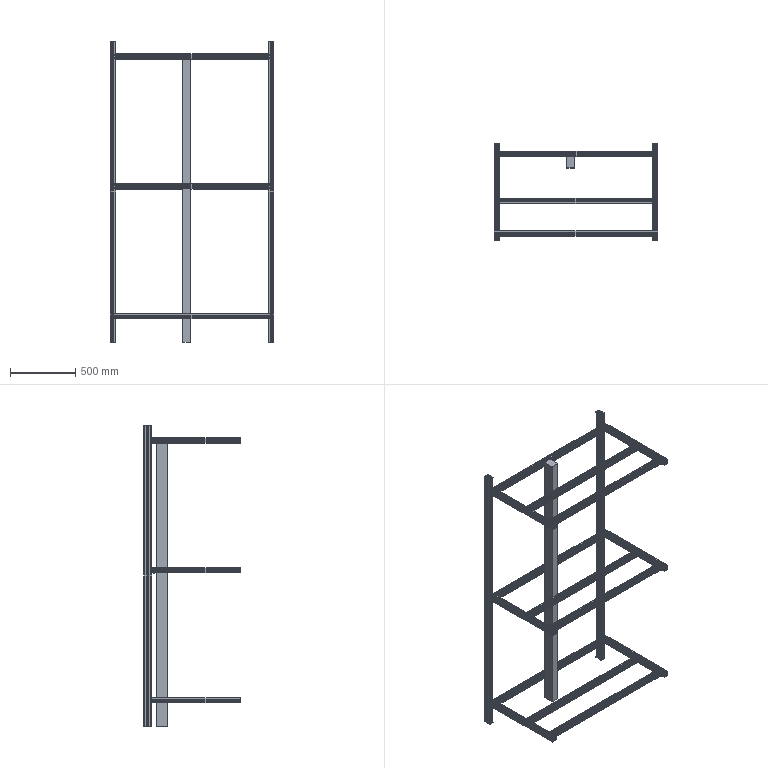Part | SolidWorks | features ICE 4, Extrusion 1, HoleWzd 1, LPattern 1 | 18 solids | 2644 faces | box 1250 x 740 x 2300 mm | volume 23808446 mm3 | plane 1948 | cylinder 696 | commonest cylinder face diameters 1 x300 9 x168 10.2 x120 6.8 x68 15 x32 3 x8